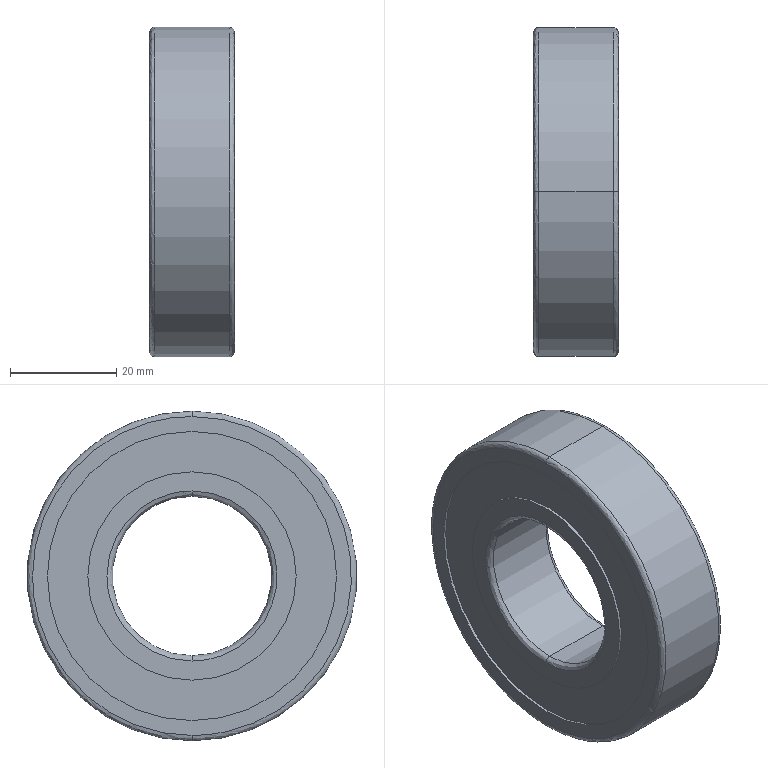Part | STEP file | 0229_009_B6206ZZ | 1 solid | 26 faces | box 16 x 62 x 62 mm | volume 35690 mm3 | cylinder 12 | spline 8 | plane 6 | commonest cylinder face diameters 39.2 x4 54.4 x4 30 x2 62 x2